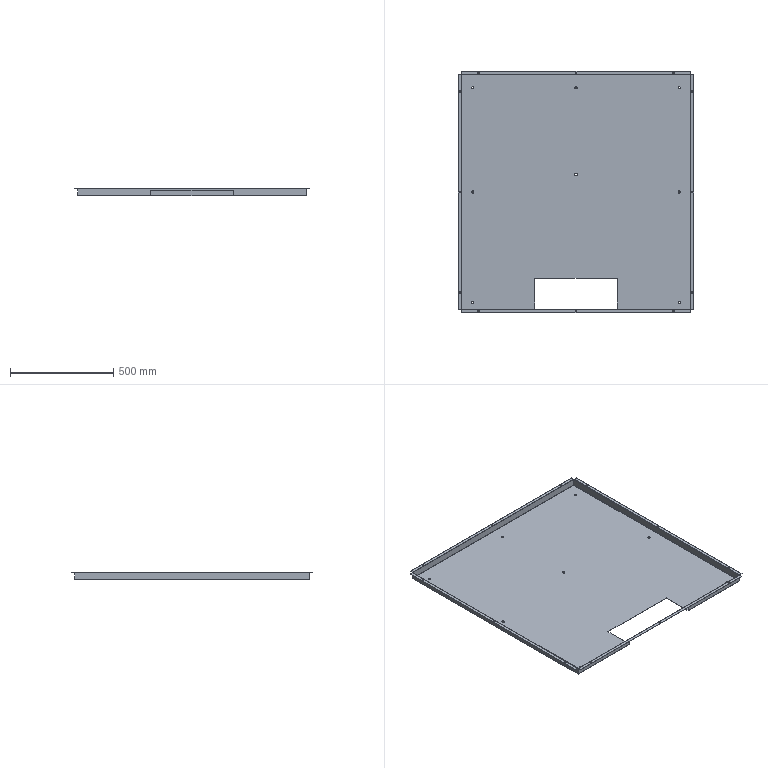Part | 1 solid | 150 faces | box 1140 x 1170 x 35 mm | volume 1410594 mm3 | plane 78 | cylinder 64 | spline 8 | commonest cylinder face diameters 7 x30 11 x16 0.4 x9 2.4 x9